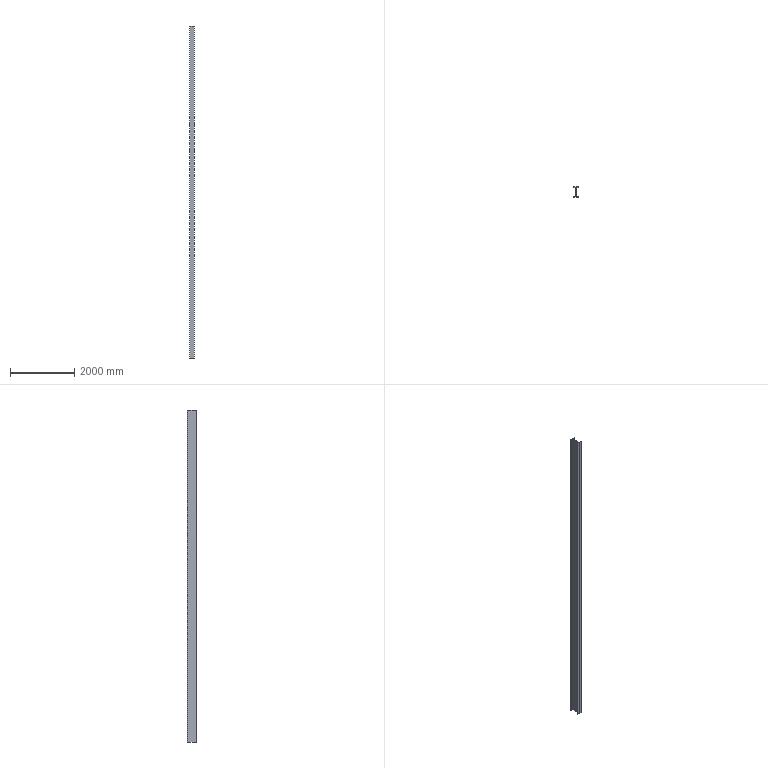Part | SolidWorks | features Extrusion 1 | 1 solid | 18 faces | box 150 x 300 x 10347 mm | volume 48403999 mm3 | plane 14 | cylinder 4 | commonest cylinder face diameters 26 x4
STEP:
#1=CARTESIAN_POINT('',(-75.,9.,0.));
#2=VERTEX_POINT('',#1);
#3=CARTESIAN_POINT('',(-75.,0.,0.));
#4=VERTEX_POINT('',#3);
#5=CARTESIAN_POINT('',(-75.,0.,0.));
#6=DIRECTION('',(0.,-1.,0.));
#7=VECTOR('',#6,1000.);
#8=LINE('',#5,#7);
#9=EDGE_CURVE('',#2,#4,#8,.T.);
#10=ORIENTED_EDGE('',*,*,#9,.T.);
#11=CARTESIAN_POINT('',(-75.,0.,10347.));
#12=VERTEX_POINT('',#11);
#13=CARTESIAN_POINT('',(-75.,0.,10347.));
#14=DIRECTION('',(0.,0.,-1.));
#15=VECTOR('',#14,1000.);
#16=LINE('',#13,#15);
#17=EDGE_CURVE('',#12,#4,#16,.T.);
#18=ORIENTED_EDGE('',*,*,#17,.F.);
#19=CARTESIAN_POINT('',(-75.,9.,10347.));
#20=VERTEX_POINT('',#19);
#21=CARTESIAN_POINT('',(-75.,0.,10347.));
#22=DIRECTION('',(0.,-1.,0.));
#23=VECTOR('',#22,1000.);
#24=LINE('',#21,#23);
#25=EDGE_CURVE('',#20,#12,#24,.T.);
#26=ORIENTED_EDGE('',*,*,#25,.F.);
#27=CARTESIAN_POINT('',(-75.,9.,10347.));
#28=DIRECTION('',(0.,0.,-1.));
#29=VECTOR('',#28,1000.);
#30=LINE('',#27,#29);
#31=EDGE_CURVE('',#20,#2,#30,.T.);
#32=ORIENTED_EDGE('',*,*,#31,.T.);
#33=EDGE_LOOP('',(#10,#18,#26,#32));
#34=FACE_OUTER_BOUND('',#33,.T.);
#35=CARTESIAN_POINT('',(-75.,0.,10347.));
#36=DIRECTION('',(1.,0.,0.));
#37=DIRECTION('',(0.,0.,-1.));
#38=AXIS2_PLACEMENT_3D('',#35,#36,#37);
#39=PLANE('',#38);
#40=ADVANCED_FACE('',(#34),#39,.F.);
#41=CARTESIAN_POINT('',(75.,0.,0.));
#42=VERTEX_POINT('',#41);
#43=CARTESIAN_POINT('',(75.,0.,0.));
#44=DIRECTION('',(1.,0.,0.));
#45=VECTOR('',#44,1000.);
#46=LINE('',#43,#45);
#47=EDGE_CURVE('',#4,#42,#46,.T.);
#48=ORIENTED_EDGE('',*,*,#47,.T.);
#49=CARTESIAN_POINT('',(75.,0.,10347.));
#50=VERTEX_POINT('',#49);
#51=CARTESIAN_POINT('',(75.,0.,10347.));
#52=DIRECTION('',(0.,0.,-1.));
#53=VECTOR('',#52,1000.);
#54=LINE('',#51,#53);
#55=EDGE_CURVE('',#50,#42,#54,.T.);
#56=ORIENTED_EDGE('',*,*,#55,.F.);
#57=CARTESIAN_POINT('',(75.,0.,10347.));
#58=DIRECTION('',(1.,0.,0.));
#59=VECTOR('',#58,1000.);
#60=LINE('',#57,#59);
#61=EDGE_CURVE('',#12,#50,#60,.T.);
#62=ORIENTED_EDGE('',*,*,#61,.F.);
#63=ORIENTED_EDGE('',*,*,#17,.T.);
#64=EDGE_LOOP('',(#48,#56,#62,#63));
#65=FACE_OUTER_BOUND('',#64,.T.);
#66=CARTESIAN_POINT('',(75.,0.,10347.));
#67=DIRECTION('',(0.,1.,0.));
#68=DIRECTION('',(-1.,0.,0.));
#69=AXIS2_PLACEMENT_3D('',#66,#67,#68);
#70=PLANE('',#69);
#71=ADVANCED_FACE('',(#65),#70,.F.);
#72=CARTESIAN_POINT('',(75.,9.,0.));
#73=VERTEX_POINT('',#72);
#74=CARTESIAN_POINT('',(75.,0.,0.));
#75=DIRECTION('',(0.,1.,0.));
#76=VECTOR('',#75,1000.);
#77=LINE('',#74,#76);
#78=EDGE_CURVE('',#42,#73,#77,.T.);
#79=ORIENTED_EDGE('',*,*,#78,.T.);
#80=CARTESIAN_POINT('',(75.,9.,10347.));
#81=VERTEX_POINT('',#80);
#82=CARTESIAN_POINT('',(75.,9.,10347.));
#83=DIRECTION('',(0.,0.,-1.));
#84=VECTOR('',#83,1000.);
#85=LINE('',#82,#84);
#86=EDGE_CURVE('',#81,#73,#85,.T.);
#87=ORIENTED_EDGE('',*,*,#86,.F.);
#88=CARTESIAN_POINT('',(75.,0.,10347.));
#89=DIRECTION('',(0.,1.,0.));
#90=VECTOR('',#89,1000.);
#91=LINE('',#88,#90);
#92=EDGE_CURVE('',#50,#81,#91,.T.);
#93=ORIENTED_EDGE('',*,*,#92,.F.);
#94=ORIENTED_EDGE('',*,*,#55,.T.);
#95=EDGE_LOOP('',(#79,#87,#93,#94));
#96=FACE_OUTER_BOUND('',#95,.T.);
#97=CARTESIAN_POINT('',(75.,0.,10347.));
#98=DIRECTION('',(-1.,0.,0.));
#99=DIRECTION('',(0.,0.,1.));
#100=AXIS2_PLACEMENT_3D('',#97,#98,#99);
#101=PLANE('',#100);
#102=ADVANCED_FACE('',(#96),#101,.F.);
#103=CARTESIAN_POINT('',(16.25,9.,0.));
#104=VERTEX_POINT('',#103);
#105=CARTESIAN_POINT('',(75.,9.,0.));
#106=DIRECTION('',(-1.,0.,0.));
#107=VECTOR('',#106,1000.);
#108=LINE('',#105,#107);
#109=EDGE_CURVE('',#73,#104,#108,.T.);
#110=ORIENTED_EDGE('',*,*,#109,.T.);
#111=CARTESIAN_POINT('',(16.25,9.,10347.));
#112=VERTEX_POINT('',#111);
#113=CARTESIAN_POINT('',(16.25,9.,10347.));
#114=DIRECTION('',(0.,0.,-1.));
#115=VECTOR('',#114,1000.);
#116=LINE('',#113,#115);
#117=EDGE_CURVE('',#112,#104,#116,.T.);
#118=ORIENTED_EDGE('',*,*,#117,.F.);
#119=CARTESIAN_POINT('',(75.,9.,10347.));
#120=DIRECTION('',(-1.,0.,0.));
#121=VECTOR('',#120,1000.);
#122=LINE('',#119,#121);
#123=EDGE_CURVE('',#81,#112,#122,.T.);
#124=ORIENTED_EDGE('',*,*,#123,.F.);
#125=ORIENTED_EDGE('',*,*,#86,.T.);
#126=EDGE_LOOP('',(#110,#118,#124,#125));
#127=FACE_OUTER_BOUND('',#126,.T.);
#128=CARTESIAN_POINT('',(75.,9.,10347.));
#129=DIRECTION('',(0.,-1.,0.));
#130=DIRECTION('',(1.,0.,0.));
#131=AXIS2_PLACEMENT_3D('',#128,#129,#130);
#132=PLANE('',#131);
#133=ADVANCED_FACE('',(#127),#132,.F.);
#134=CARTESIAN_POINT('',(3.25,22.,0.));
#135=VERTEX_POINT('',#134);
#136=CARTESIAN_POINT('',(16.25,22.,0.));
#137=DIRECTION('',(0.,0.,-1.));
#138=DIRECTION('',(-1.,0.,0.));
#139=AXIS2_PLACEMENT_3D('',#136,#137,#138);
#140=CIRCLE('',#139,13.);
#141=EDGE_CURVE('',#104,#135,#140,.T.);
#142=ORIENTED_EDGE('',*,*,#141,.T.);
#143=CARTESIAN_POINT('',(3.25,22.,10347.));
#144=VERTEX_POINT('',#143);
#145=CARTESIAN_POINT('',(3.25,22.,10347.));
#146=DIRECTION('',(0.,0.,-1.));
#147=VECTOR('',#146,1000.);
#148=LINE('',#145,#147);
#149=EDGE_CURVE('',#144,#135,#148,.T.);
#150=ORIENTED_EDGE('',*,*,#149,.F.);
#151=CARTESIAN_POINT('',(16.25,22.,10347.));
#152=DIRECTION('',(0.,0.,-1.));
#153=DIRECTION('',(-1.,0.,0.));
#154=AXIS2_PLACEMENT_3D('',#151,#152,#153);
#155=CIRCLE('',#154,13.);
#156=EDGE_CURVE('',#112,#144,#155,.T.);
#157=ORIENTED_EDGE('',*,*,#156,.F.);
#158=ORIENTED_EDGE('',*,*,#117,.T.);
#159=EDGE_LOOP('',(#142,#150,#157,#158));
#160=FACE_OUTER_BOUND('',#159,.T.);
#161=CARTESIAN_POINT('',(16.25,22.,10347.));
#162=DIRECTION('',(0.,0.,-1.));
#163=DIRECTION('',(-1.,0.,0.));
#164=AXIS2_PLACEMENT_3D('',#161,#162,#163);
#165=CYLINDRICAL_SURFACE('',#164,13.);
#166=ADVANCED_FACE('',(#160),#165,.F.);
#167=CARTESIAN_POINT('',(3.25,278.,0.));
#168=VERTEX_POINT('',#167);
#169=CARTESIAN_POINT('',(3.25,22.,0.));
#170=DIRECTION('',(0.,1.,0.));
#171=VECTOR('',#170,1000.);
#172=LINE('',#169,#171);
#173=EDGE_CURVE('',#135,#168,#172,.T.);
#174=ORIENTED_EDGE('',*,*,#173,.T.);
#175=CARTESIAN_POINT('',(3.25,278.,10347.));
#176=VERTEX_POINT('',#175);
#177=CARTESIAN_POINT('',(3.25,278.,10347.));
#178=DIRECTION('',(0.,0.,-1.));
#179=VECTOR('',#178,1000.);
#180=LINE('',#177,#179);
#181=EDGE_CURVE('',#176,#168,#180,.T.);
#182=ORIENTED_EDGE('',*,*,#181,.F.);
#183=CARTESIAN_POINT('',(3.25,22.,10347.));
#184=DIRECTION('',(0.,1.,0.));
#185=VECTOR('',#184,1000.);
#186=LINE('',#183,#185);
#187=EDGE_CURVE('',#144,#176,#186,.T.);
#188=ORIENTED_EDGE('',*,*,#187,.F.);
#189=ORIENTED_EDGE('',*,*,#149,.T.);
#190=EDGE_LOOP('',(#174,#182,#188,#189));
#191=FACE_OUTER_BOUND('',#190,.T.);
#192=CARTESIAN_POINT('',(3.25,22.,10347.));
#193=DIRECTION('',(-1.,0.,0.));
#194=DIRECTION('',(0.,0.,1.));
#195=AXIS2_PLACEMENT_3D('',#192,#193,#194);
#196=PLANE('',#195);
#197=ADVANCED_FACE('',(#191),#196,.F.);
#198=CARTESIAN_POINT('',(16.25,291.,0.));
#199=VERTEX_POINT('',#198);
#200=CARTESIAN_POINT('',(16.25,278.,0.));
#201=DIRECTION('',(0.,0.,-1.));
#202=DIRECTION('',(-1.,0.,0.));
#203=AXIS2_PLACEMENT_3D('',#200,#201,#202);
#204=CIRCLE('',#203,13.);
#205=EDGE_CURVE('',#168,#199,#204,.T.);
#206=ORIENTED_EDGE('',*,*,#205,.T.);
#207=CARTESIAN_POINT('',(16.25,291.,10347.));
#208=VERTEX_POINT('',#207);
#209=CARTESIAN_POINT('',(16.25,291.,10347.));
#210=DIRECTION('',(0.,0.,-1.));
#211=VECTOR('',#210,1000.);
#212=LINE('',#209,#211);
#213=EDGE_CURVE('',#208,#199,#212,.T.);
#214=ORIENTED_EDGE('',*,*,#213,.F.);
#215=CARTESIAN_POINT('',(16.25,278.,10347.));
#216=DIRECTION('',(0.,0.,-1.));
#217=DIRECTION('',(-1.,0.,0.));
#218=AXIS2_PLACEMENT_3D('',#215,#216,#217);
#219=CIRCLE('',#218,13.);
#220=EDGE_CURVE('',#176,#208,#219,.T.);
#221=ORIENTED_EDGE('',*,*,#220,.F.);
#222=ORIENTED_EDGE('',*,*,#181,.T.);
#223=EDGE_LOOP('',(#206,#214,#221,#222));
#224=FACE_OUTER_BOUND('',#223,.T.);
#225=CARTESIAN_POINT('',(16.25,278.,10347.));
#226=DIRECTION('',(0.,0.,-1.));
#227=DIRECTION('',(-1.,0.,0.));
#228=AXIS2_PLACEMENT_3D('',#225,#226,#227);
#229=CYLINDRICAL_SURFACE('',#228,13.);
#230=ADVANCED_FACE('',(#224),#229,.F.);
#231=CARTESIAN_POINT('',(75.,291.,0.));
#232=VERTEX_POINT('',#231);
#233=CARTESIAN_POINT('',(16.25,291.,0.));
#234=DIRECTION('',(1.,0.,0.));
#235=VECTOR('',#234,1000.);
#236=LINE('',#233,#235);
#237=EDGE_CURVE('',#199,#232,#236,.T.);
#238=ORIENTED_EDGE('',*,*,#237,.T.);
#239=CARTESIAN_POINT('',(75.,291.,10347.));
#240=VERTEX_POINT('',#239);
#241=CARTESIAN_POINT('',(75.,291.,10347.));
#242=DIRECTION('',(0.,0.,-1.));
#243=VECTOR('',#242,1000.);
#244=LINE('',#241,#243);
#245=EDGE_CURVE('',#240,#232,#244,.T.);
#246=ORIENTED_EDGE('',*,*,#245,.F.);
#247=CARTESIAN_POINT('',(16.25,291.,10347.));
#248=DIRECTION('',(1.,0.,0.));
#249=VECTOR('',#248,1000.);
#250=LINE('',#247,#249);
#251=EDGE_CURVE('',#208,#240,#250,.T.);
#252=ORIENTED_EDGE('',*,*,#251,.F.);
#253=ORIENTED_EDGE('',*,*,#213,.T.);
#254=EDGE_LOOP('',(#238,#246,#252,#253));
#255=FACE_OUTER_BOUND('',#254,.T.);
#256=CARTESIAN_POINT('',(16.25,291.,10347.));
#257=DIRECTION('',(0.,1.,0.));
#258=DIRECTION('',(-1.,0.,0.));
#259=AXIS2_PLACEMENT_3D('',#256,#257,#258);
#260=PLANE('',#259);
#261=ADVANCED_FACE('',(#255),#260,.F.);
#262=CARTESIAN_POINT('',(75.,300.,0.));
#263=VERTEX_POINT('',#262);
#264=CARTESIAN_POINT('',(75.,291.,0.));
#265=DIRECTION('',(0.,1.,0.));
#266=VECTOR('',#265,1000.);
#267=LINE('',#264,#266);
#268=EDGE_CURVE('',#232,#263,#267,.T.);
#269=ORIENTED_EDGE('',*,*,#268,.T.);
#270=CARTESIAN_POINT('',(75.,300.,10347.));
#271=VERTEX_POINT('',#270);
#272=CARTESIAN_POINT('',(75.,300.,10347.));
#273=DIRECTION('',(0.,0.,-1.));
#274=VECTOR('',#273,1000.);
#275=LINE('',#272,#274);
#276=EDGE_CURVE('',#271,#263,#275,.T.);
#277=ORIENTED_EDGE('',*,*,#276,.F.);
#278=CARTESIAN_POINT('',(75.,291.,10347.));
#279=DIRECTION('',(0.,1.,0.));
#280=VECTOR('',#279,1000.);
#281=LINE('',#278,#280);
#282=EDGE_CURVE('',#240,#271,#281,.T.);
#283=ORIENTED_EDGE('',*,*,#282,.F.);
#284=ORIENTED_EDGE('',*,*,#245,.T.);
#285=EDGE_LOOP('',(#269,#277,#283,#284));
#286=FACE_OUTER_BOUND('',#285,.T.);
#287=CARTESIAN_POINT('',(75.,291.,10347.));
#288=DIRECTION('',(-1.,0.,0.));
#289=DIRECTION('',(0.,-1.,0.));
#290=AXIS2_PLACEMENT_3D('',#287,#288,#289);
#291=PLANE('',#290);
#292=ADVANCED_FACE('',(#286),#291,.F.);
#293=CARTESIAN_POINT('',(-75.,300.,0.));
#294=VERTEX_POINT('',#293);
#295=CARTESIAN_POINT('',(-75.,300.,0.));
#296=DIRECTION('',(-1.,0.,0.));
#297=VECTOR('',#296,1000.);
#298=LINE('',#295,#297);
#299=EDGE_CURVE('',#263,#294,#298,.T.);
#300=ORIENTED_EDGE('',*,*,#299,.T.);
#301=CARTESIAN_POINT('',(-75.,300.,10347.));
#302=VERTEX_POINT('',#301);
#303=CARTESIAN_POINT('',(-75.,300.,10347.));
#304=DIRECTION('',(0.,0.,-1.));
#305=VECTOR('',#304,1000.);
#306=LINE('',#303,#305);
#307=EDGE_CURVE('',#302,#294,#306,.T.);
#308=ORIENTED_EDGE('',*,*,#307,.F.);
#309=CARTESIAN_POINT('',(-75.,300.,10347.));
#310=DIRECTION('',(-1.,0.,0.));
#311=VECTOR('',#310,1000.);
#312=LINE('',#309,#311);
#313=EDGE_CURVE('',#271,#302,#312,.T.);
#314=ORIENTED_EDGE('',*,*,#313,.F.);
#315=ORIENTED_EDGE('',*,*,#276,.T.);
#316=EDGE_LOOP('',(#300,#308,#314,#315));
#317=FACE_OUTER_BOUND('',#316,.T.);
#318=CARTESIAN_POINT('',(-75.,300.,10347.));
#319=DIRECTION('',(0.,-1.,0.));
#320=DIRECTION('',(0.,0.,-1.));
#321=AXIS2_PLACEMENT_3D('',#318,#319,#320);
#322=PLANE('',#321);
#323=ADVANCED_FACE('',(#317),#322,.F.);
#324=CARTESIAN_POINT('',(-75.,291.,0.));
#325=VERTEX_POINT('',#324);
#326=CARTESIAN_POINT('',(-75.,291.,0.));
#327=DIRECTION('',(0.,-1.,0.));
#328=VECTOR('',#327,1000.);
#329=LINE('',#326,#328);
#330=EDGE_CURVE('',#294,#325,#329,.T.);
#331=ORIENTED_EDGE('',*,*,#330,.T.);
#332=CARTESIAN_POINT('',(-75.,291.,10347.));
#333=VERTEX_POINT('',#332);
#334=CARTESIAN_POINT('',(-75.,291.,10347.));
#335=DIRECTION('',(0.,0.,-1.));
#336=VECTOR('',#335,1000.);
#337=LINE('',#334,#336);
#338=EDGE_CURVE('',#333,#325,#337,.T.);
#339=ORIENTED_EDGE('',*,*,#338,.F.);
#340=CARTESIAN_POINT('',(-75.,291.,10347.));
#341=DIRECTION('',(0.,-1.,0.));
#342=VECTOR('',#341,1000.);
#343=LINE('',#340,#342);
#344=EDGE_CURVE('',#302,#333,#343,.T.);
#345=ORIENTED_EDGE('',*,*,#344,.F.);
#346=ORIENTED_EDGE('',*,*,#307,.T.);
#347=EDGE_LOOP('',(#331,#339,#345,#346));
#348=FACE_OUTER_BOUND('',#347,.T.);
#349=CARTESIAN_POINT('',(-75.,291.,10347.));
#350=DIRECTION('',(1.,0.,0.));
#351=DIRECTION('',(0.,1.,0.));
#352=AXIS2_PLACEMENT_3D('',#349,#350,#351);
#353=PLANE('',#352);
#354=ADVANCED_FACE('',(#348),#353,.F.);
#355=CARTESIAN_POINT('',(-16.25,291.,0.));
#356=VERTEX_POINT('',#355);
#357=CARTESIAN_POINT('',(-16.25,291.,0.));
#358=DIRECTION('',(1.,0.,0.));
#359=VECTOR('',#358,1000.);
#360=LINE('',#357,#359);
#361=EDGE_CURVE('',#325,#356,#360,.T.);
#362=ORIENTED_EDGE('',*,*,#361,.T.);
#363=CARTESIAN_POINT('',(-16.25,291.,10347.));
#364=VERTEX_POINT('',#363);
#365=CARTESIAN_POINT('',(-16.25,291.,10347.));
#366=DIRECTION('',(0.,0.,-1.));
#367=VECTOR('',#366,1000.);
#368=LINE('',#365,#367);
#369=EDGE_CURVE('',#364,#356,#368,.T.);
#370=ORIENTED_EDGE('',*,*,#369,.F.);
#371=CARTESIAN_POINT('',(-16.25,291.,10347.));
#372=DIRECTION('',(1.,0.,0.));
#373=VECTOR('',#372,1000.);
#374=LINE('',#371,#373);
#375=EDGE_CURVE('',#333,#364,#374,.T.);
#376=ORIENTED_EDGE('',*,*,#375,.F.);
#377=ORIENTED_EDGE('',*,*,#338,.T.);
#378=EDGE_LOOP('',(#362,#370,#376,#377));
#379=FACE_OUTER_BOUND('',#378,.T.);
#380=CARTESIAN_POINT('',(-16.25,291.,10347.));
#381=DIRECTION('',(0.,1.,0.));
#382=DIRECTION('',(-1.,0.,0.));
#383=AXIS2_PLACEMENT_3D('',#380,#381,#382);
#384=PLANE('',#383);
#385=ADVANCED_FACE('',(#379),#384,.F.);
#386=CARTESIAN_POINT('',(-3.25,278.,0.));
#387=VERTEX_POINT('',#386);
#388=CARTESIAN_POINT('',(-16.25,278.,0.));
#389=DIRECTION('',(0.,0.,-1.));
#390=DIRECTION('',(1.,0.,0.));
#391=AXIS2_PLACEMENT_3D('',#388,#389,#390);
#392=CIRCLE('',#391,13.);
#393=EDGE_CURVE('',#356,#387,#392,.T.);
#394=ORIENTED_EDGE('',*,*,#393,.T.);
#395=CARTESIAN_POINT('',(-3.25,278.,10347.));
#396=VERTEX_POINT('',#395);
#397=CARTESIAN_POINT('',(-3.25,278.,10347.));
#398=DIRECTION('',(0.,0.,-1.));
#399=VECTOR('',#398,1000.);
#400=LINE('',#397,#399);
#401=EDGE_CURVE('',#396,#387,#400,.T.);
#402=ORIENTED_EDGE('',*,*,#401,.F.);
#403=CARTESIAN_POINT('',(-16.25,278.,10347.));
#404=DIRECTION('',(0.,0.,-1.));
#405=DIRECTION('',(1.,0.,0.));
#406=AXIS2_PLACEMENT_3D('',#403,#404,#405);
#407=CIRCLE('',#406,13.);
#408=EDGE_CURVE('',#364,#396,#407,.T.);
#409=ORIENTED_EDGE('',*,*,#408,.F.);
#410=ORIENTED_EDGE('',*,*,#369,.T.);
#411=EDGE_LOOP('',(#394,#402,#409,#410));
#412=FACE_OUTER_BOUND('',#411,.T.);
#413=CARTESIAN_POINT('',(-16.25,278.,10347.));
#414=DIRECTION('',(0.,0.,-1.));
#415=DIRECTION('',(-1.,0.,0.));
#416=AXIS2_PLACEMENT_3D('',#413,#414,#415);
#417=CYLINDRICAL_SURFACE('',#416,13.);
#418=ADVANCED_FACE('',(#412),#417,.F.);
#419=CARTESIAN_POINT('',(-3.25,22.,0.));
#420=VERTEX_POINT('',#419);
#421=CARTESIAN_POINT('',(-3.25,22.,0.));
#422=DIRECTION('',(0.,-1.,0.));
#423=VECTOR('',#422,1000.);
#424=LINE('',#421,#423);
#425=EDGE_CURVE('',#387,#420,#424,.T.);
#426=ORIENTED_EDGE('',*,*,#425,.T.);
#427=CARTESIAN_POINT('',(-3.25,22.,10347.));
#428=VERTEX_POINT('',#427);
#429=CARTESIAN_POINT('',(-3.25,22.,10347.));
#430=DIRECTION('',(0.,0.,-1.));
#431=VECTOR('',#430,1000.);
#432=LINE('',#429,#431);
#433=EDGE_CURVE('',#428,#420,#432,.T.);
#434=ORIENTED_EDGE('',*,*,#433,.F.);
#435=CARTESIAN_POINT('',(-3.25,22.,10347.));
#436=DIRECTION('',(0.,-1.,0.));
#437=VECTOR('',#436,1000.);
#438=LINE('',#435,#437);
#439=EDGE_CURVE('',#396,#428,#438,.T.);
#440=ORIENTED_EDGE('',*,*,#439,.F.);
#441=ORIENTED_EDGE('',*,*,#401,.T.);
#442=EDGE_LOOP('',(#426,#434,#440,#441));
#443=FACE_OUTER_BOUND('',#442,.T.);
#444=CARTESIAN_POINT('',(-3.25,22.,10347.));
#445=DIRECTION('',(1.,0.,0.));
#446=DIRECTION('',(0.,0.,-1.));
#447=AXIS2_PLACEMENT_3D('',#444,#445,#446);
#448=PLANE('',#447);
#449=ADVANCED_FACE('',(#443),#448,.F.);
#450=CARTESIAN_POINT('',(-16.25,9.,0.));
#451=VERTEX_POINT('',#450);
#452=CARTESIAN_POINT('',(-16.25,22.,0.));
#453=DIRECTION('',(0.,0.,-1.));
#454=DIRECTION('',(-1.,0.,0.));
#455=AXIS2_PLACEMENT_3D('',#452,#453,#454);
#456=CIRCLE('',#455,13.);
#457=EDGE_CURVE('',#420,#451,#456,.T.);
#458=ORIENTED_EDGE('',*,*,#457,.T.);
#459=CARTESIAN_POINT('',(-16.25,9.,10347.));
#460=VERTEX_POINT('',#459);
#461=CARTESIAN_POINT('',(-16.25,9.,10347.));
#462=DIRECTION('',(0.,0.,-1.));
#463=VECTOR('',#462,1000.);
#464=LINE('',#461,#463);
#465=EDGE_CURVE('',#460,#451,#464,.T.);
#466=ORIENTED_EDGE('',*,*,#465,.F.);
#467=CARTESIAN_POINT('',(-16.25,22.,10347.));
#468=DIRECTION('',(0.,0.,-1.));
#469=DIRECTION('',(-1.,0.,0.));
#470=AXIS2_PLACEMENT_3D('',#467,#468,#469);
#471=CIRCLE('',#470,13.);
#472=EDGE_CURVE('',#428,#460,#471,.T.);
#473=ORIENTED_EDGE('',*,*,#472,.F.);
#474=ORIENTED_EDGE('',*,*,#433,.T.);
#475=EDGE_LOOP('',(#458,#466,#473,#474));
#476=FACE_OUTER_BOUND('',#475,.T.);
#477=CARTESIAN_POINT('',(-16.25,22.,10347.));
#478=DIRECTION('',(0.,0.,-1.));
#479=DIRECTION('',(-1.,0.,0.));
#480=AXIS2_PLACEMENT_3D('',#477,#478,#479);
#481=CYLINDRICAL_SURFACE('',#480,13.);
#482=ADVANCED_FACE('',(#476),#481,.F.);
#483=CARTESIAN_POINT('',(-75.,9.,0.));
#484=DIRECTION('',(-1.,0.,0.));
#485=VECTOR('',#484,1000.);
#486=LINE('',#483,#485);
#487=EDGE_CURVE('',#451,#2,#486,.T.);
#488=ORIENTED_EDGE('',*,*,#487,.T.);
#489=ORIENTED_EDGE('',*,*,#31,.F.);
#490=CARTESIAN_POINT('',(-75.,9.,10347.));
#491=DIRECTION('',(-1.,0.,0.));
#492=VECTOR('',#491,1000.);
#493=LINE('',#490,#492);
#494=EDGE_CURVE('',#460,#20,#493,.T.);
#495=ORIENTED_EDGE('',*,*,#494,.F.);
#496=ORIENTED_EDGE('',*,*,#465,.T.);
#497=EDGE_LOOP('',(#488,#489,#495,#496));
#498=FACE_OUTER_BOUND('',#497,.T.);
#499=CARTESIAN_POINT('',(-75.,9.,10347.));
#500=DIRECTION('',(0.,-1.,0.));
#501=DIRECTION('',(1.,0.,0.));
#502=AXIS2_PLACEMENT_3D('',#499,#500,#501);
#503=PLANE('',#502);
#504=ADVANCED_FACE('',(#498),#503,.F.);
#505=ORIENTED_EDGE('',*,*,#25,.T.);
#506=ORIENTED_EDGE('',*,*,#61,.T.);
#507=ORIENTED_EDGE('',*,*,#92,.T.);
#508=ORIENTED_EDGE('',*,*,#123,.T.);
#509=ORIENTED_EDGE('',*,*,#156,.T.);
#510=ORIENTED_EDGE('',*,*,#187,.T.);
#511=ORIENTED_EDGE('',*,*,#220,.T.);
#512=ORIENTED_EDGE('',*,*,#251,.T.);
#513=ORIENTED_EDGE('',*,*,#282,.T.);
#514=ORIENTED_EDGE('',*,*,#313,.T.);
#515=ORIENTED_EDGE('',*,*,#344,.T.);
#516=ORIENTED_EDGE('',*,*,#375,.T.);
#517=ORIENTED_EDGE('',*,*,#408,.T.);
#518=ORIENTED_EDGE('',*,*,#439,.T.);
#519=ORIENTED_EDGE('',*,*,#472,.T.);
#520=ORIENTED_EDGE('',*,*,#494,.T.);
#521=EDGE_LOOP('',(#505,#506,#507,#508,#509,#510,#511,#512,#513,#514,#515,#516,#517,#518,#519,#520));
#522=FACE_OUTER_BOUND('',#521,.T.);
#523=CARTESIAN_POINT('',(-16.25,22.,10347.));
#524=DIRECTION('',(0.,0.,-1.));
#525=DIRECTION('',(-1.,0.,0.));
#526=AXIS2_PLACEMENT_3D('',#523,#524,#525);
#527=PLANE('',#526);
#528=ADVANCED_FACE('',(#522),#527,.F.);
#529=ORIENTED_EDGE('',*,*,#9,.F.);
#530=ORIENTED_EDGE('',*,*,#487,.F.);
#531=ORIENTED_EDGE('',*,*,#457,.F.);
#532=ORIENTED_EDGE('',*,*,#425,.F.);
#533=ORIENTED_EDGE('',*,*,#393,.F.);
#534=ORIENTED_EDGE('',*,*,#361,.F.);
#535=ORIENTED_EDGE('',*,*,#330,.F.);
#536=ORIENTED_EDGE('',*,*,#299,.F.);
#537=ORIENTED_EDGE('',*,*,#268,.F.);
#538=ORIENTED_EDGE('',*,*,#237,.F.);
#539=ORIENTED_EDGE('',*,*,#205,.F.);
#540=ORIENTED_EDGE('',*,*,#173,.F.);
#541=ORIENTED_EDGE('',*,*,#141,.F.);
#542=ORIENTED_EDGE('',*,*,#109,.F.);
#543=ORIENTED_EDGE('',*,*,#78,.F.);
#544=ORIENTED_EDGE('',*,*,#47,.F.);
#545=EDGE_LOOP('',(#529,#530,#531,#532,#533,#534,#535,#536,#537,#538,#539,#540,#541,#542,#543,#544));
#546=FACE_OUTER_BOUND('',#545,.T.);
#547=CARTESIAN_POINT('',(-16.25,22.,0.));
#548=DIRECTION('',(0.,0.,-1.));
#549=DIRECTION('',(-1.,0.,0.));
#550=AXIS2_PLACEMENT_3D('',#547,#548,#549);
#551=PLANE('',#550);
#552=ADVANCED_FACE('',(#546),#551,.T.);
#553=CLOSED_SHELL('',(#40,#71,#102,#133,#166,#197,#230,#261,#292,#323,#354,#385,#418,#449,#482,#504,#528,#552));
#554=MANIFOLD_SOLID_BREP('',#553);
#555=CARTESIAN_POINT('',(0.,0.,0.));
#556=DIRECTION('',(0.,0.,1.));
#557=DIRECTION('',(1.,0.,0.));
#558=AXIS2_PLACEMENT_3D('',#555,#556,#557);
#559=(LENGTH_UNIT()NAMED_UNIT(*)SI_UNIT(.MILLI.,.METRE.));
#560=UNCERTAINTY_MEASURE_WITH_UNIT(LENGTH_MEASURE(0.00001),#559,'','');
#561=(NAMED_UNIT(*)PLANE_ANGLE_UNIT()SI_UNIT($,.RADIAN.));
#562=(NAMED_UNIT(*)SI_UNIT($,.STERADIAN.)SOLID_ANGLE_UNIT());
#563=(GEOMETRIC_REPRESENTATION_CONTEXT(3)GLOBAL_UNCERTAINTY_ASSIGNED_CONTEXT((#560))GLOBAL_UNIT_ASSIGNED_CONTEXT((#559,#561,#562))REPRESENTATION_CONTEXT('',''));
#564=ADVANCED_BREP_SHAPE_REPRESENTATION('',(#554,#558),#563);